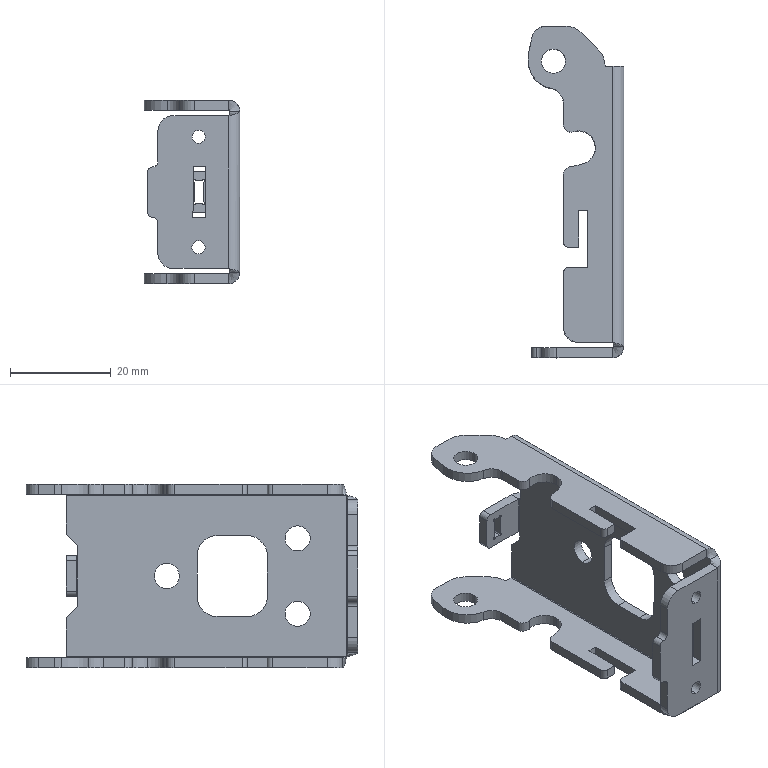Part | SolidWorks | features BaseBody 1 | 1 solid | 143 faces | box 19.031 x 66.015 x 36.541 mm | volume 6772 mm3 | plane 70 | cylinder 69 | spline 4 | commonest cylinder face diameters 2 x10 6 x8 0.5 x7 5 x6 0.4 x4 2.632 x4